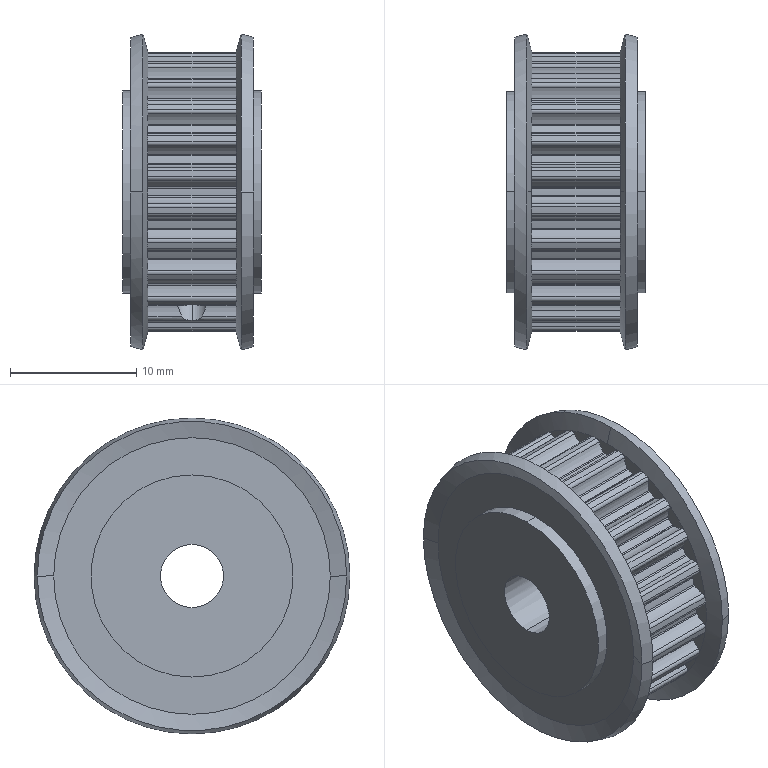Part | NX | features BREP 3 | 3 solids | 346 faces | box 11 x 25 x 25 mm | volume 3536 mm3 | cylinder 242 | plane 80 | cone 24 | commonest cylinder face diameters 0.56 x63 0.3 x58 3.95 x56 19.94 x27 22.16 x24 2.459 x4